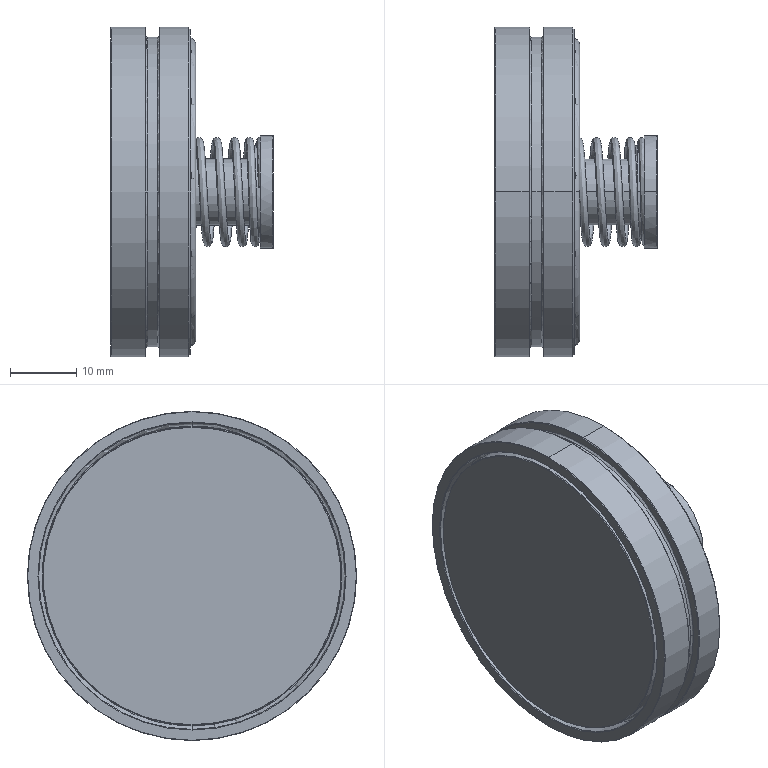Part | NX | features BREP 3 | 3 solids | 651 faces | box 24.5 x 49.6 x 49.6 mm | volume 19242 mm3 | cylinder 299 | spline 250 | plane 43 | cone 41 | torus 18 | commonest cylinder face diameters 3.3 x66 4.015 x66 0.4 x56 1.3 x32 42.6 x13 46.4 x13